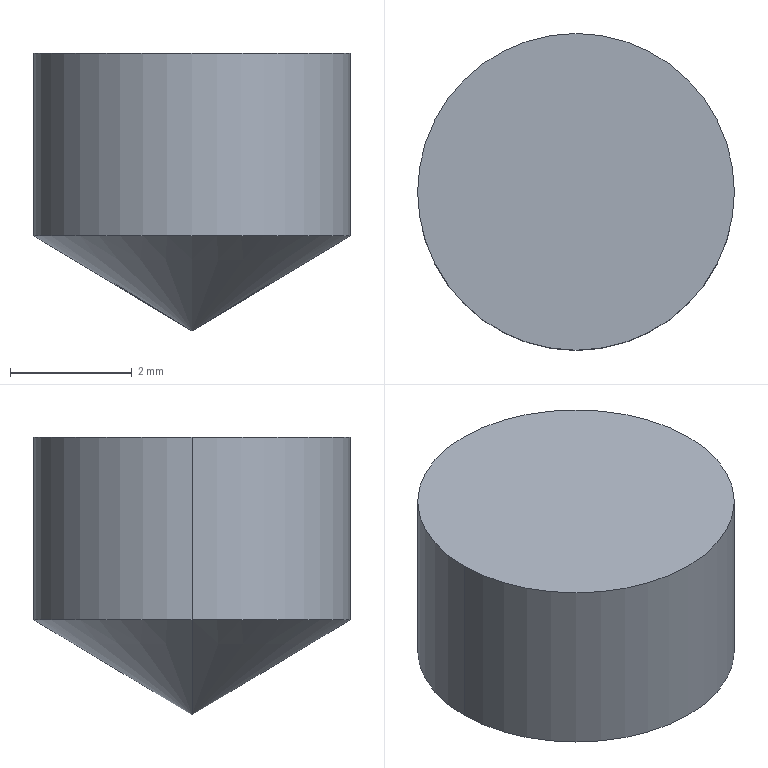Part | SolidWorks | features BaseBody 1 | 1 solid | 5 faces | box 5.2 x 5.2 x 4.562 mm | volume 74.771 mm3 | cylinder 2 | cone 2 | plane 1 | commonest cylinder face diameters 5.2 x2
STEP:
#1=CARTESIAN_POINT('',(-227.35,-157.5,81.));
#2=VERTEX_POINT('',#1);
#3=CARTESIAN_POINT('',(-222.15,-157.5,81.));
#4=VERTEX_POINT('',#3);
#5=CARTESIAN_POINT('',(-224.75,-157.5,81.));
#6=DIRECTION('',(0.,0.,-1.));
#7=DIRECTION('',(-1.,0.,0.));
#8=AXIS2_PLACEMENT_3D('',#5,#6,#7);
#9=CIRCLE('',#8,2.6);
#10=EDGE_CURVE('',#2,#4,#9,.T.);
#11=ORIENTED_EDGE('',*,*,#10,.T.);
#12=CARTESIAN_POINT('',(-222.15,-157.5,78.));
#13=VERTEX_POINT('',#12);
#14=CARTESIAN_POINT('',(-222.15,-157.5,94.));
#15=DIRECTION('',(0.,0.,-1.));
#16=VECTOR('',#15,1000.);
#17=LINE('',#14,#16);
#18=EDGE_CURVE('',#4,#13,#17,.T.);
#19=ORIENTED_EDGE('',*,*,#18,.T.);
#20=CARTESIAN_POINT('',(-227.35,-157.5,78.));
#21=VERTEX_POINT('',#20);
#22=CARTESIAN_POINT('',(-224.75,-157.5,78.));
#23=DIRECTION('',(0.,0.,1.));
#24=DIRECTION('',(-1.,0.,0.));
#25=AXIS2_PLACEMENT_3D('',#22,#23,#24);
#26=CIRCLE('',#25,2.6);
#27=EDGE_CURVE('',#13,#21,#26,.T.);
#28=ORIENTED_EDGE('',*,*,#27,.T.);
#29=CARTESIAN_POINT('',(-227.35,-157.5,94.));
#30=DIRECTION('',(0.,0.,-1.));
#31=VECTOR('',#30,1000.);
#32=LINE('',#29,#31);
#33=EDGE_CURVE('',#2,#21,#32,.T.);
#34=ORIENTED_EDGE('',*,*,#33,.F.);
#35=EDGE_LOOP('',(#11,#19,#28,#34));
#36=FACE_OUTER_BOUND('',#35,.T.);
#37=CARTESIAN_POINT('',(-224.75,-157.5,94.));
#38=DIRECTION('',(0.,0.,-1.));
#39=DIRECTION('',(-1.,0.,0.));
#40=AXIS2_PLACEMENT_3D('',#37,#38,#39);
#41=CYLINDRICAL_SURFACE('',#40,2.6);
#42=ADVANCED_FACE('',(#36),#41,.T.);
#43=CARTESIAN_POINT('',(-224.75,-157.5,76.438));
#44=VERTEX_POINT('',#43);
#45=CARTESIAN_POINT('',(-222.15,-157.5,78.));
#46=DIRECTION('',(0.8572,0.,0.515));
#47=VECTOR('',#46,1000.);
#48=LINE('',#45,#47);
#49=EDGE_CURVE('',#44,#13,#48,.T.);
#50=ORIENTED_EDGE('',*,*,#49,.F.);
#51=CARTESIAN_POINT('',(-227.35,-157.5,78.));
#52=DIRECTION('',(-0.8572,0.,0.515));
#53=VECTOR('',#52,1000.);
#54=LINE('',#51,#53);
#55=EDGE_CURVE('',#44,#21,#54,.T.);
#56=ORIENTED_EDGE('',*,*,#55,.T.);
#57=ORIENTED_EDGE('',*,*,#27,.F.);
#58=EDGE_LOOP('',(#50,#56,#57));
#59=FACE_OUTER_BOUND('',#58,.T.);
#60=CARTESIAN_POINT('',(-224.75,-157.5,78.));
#61=DIRECTION('',(0.,0.,1.));
#62=DIRECTION('',(1.,0.,0.));
#63=AXIS2_PLACEMENT_3D('',#60,#61,#62);
#64=CONICAL_SURFACE('',#63,2.6,1.03);
#65=ADVANCED_FACE('',(#59),#64,.T.);
#66=ORIENTED_EDGE('',*,*,#10,.F.);
#67=CARTESIAN_POINT('',(-224.75,-157.5,81.));
#68=DIRECTION('',(0.,0.,-1.));
#69=DIRECTION('',(-1.,0.,0.));
#70=AXIS2_PLACEMENT_3D('',#67,#68,#69);
#71=CIRCLE('',#70,2.6);
#72=EDGE_CURVE('',#4,#2,#71,.T.);
#73=ORIENTED_EDGE('',*,*,#72,.F.);
#74=EDGE_LOOP('',(#66,#73));
#75=FACE_OUTER_BOUND('',#74,.T.);
#76=CARTESIAN_POINT('',(-221.9,-4.,81.));
#77=DIRECTION('',(0.,0.,1.));
#78=DIRECTION('',(1.,0.,0.));
#79=AXIS2_PLACEMENT_3D('',#76,#77,#78);
#80=PLANE('',#79);
#81=ADVANCED_FACE('',(#75),#80,.T.);
#82=ORIENTED_EDGE('',*,*,#55,.F.);
#83=ORIENTED_EDGE('',*,*,#49,.T.);
#84=CARTESIAN_POINT('',(-224.75,-157.5,78.));
#85=DIRECTION('',(0.,0.,1.));
#86=DIRECTION('',(-1.,0.,0.));
#87=AXIS2_PLACEMENT_3D('',#84,#85,#86);
#88=CIRCLE('',#87,2.6);
#89=EDGE_CURVE('',#21,#13,#88,.T.);
#90=ORIENTED_EDGE('',*,*,#89,.F.);
#91=EDGE_LOOP('',(#82,#83,#90));
#92=FACE_OUTER_BOUND('',#91,.T.);
#93=CARTESIAN_POINT('',(-224.75,-157.5,78.));
#94=DIRECTION('',(0.,0.,1.));
#95=DIRECTION('',(1.,0.,0.));
#96=AXIS2_PLACEMENT_3D('',#93,#94,#95);
#97=CONICAL_SURFACE('',#96,2.6,1.03);
#98=ADVANCED_FACE('',(#92),#97,.T.);
#99=ORIENTED_EDGE('',*,*,#18,.F.);
#100=ORIENTED_EDGE('',*,*,#72,.T.);
#101=ORIENTED_EDGE('',*,*,#33,.T.);
#102=ORIENTED_EDGE('',*,*,#89,.T.);
#103=EDGE_LOOP('',(#99,#100,#101,#102));
#104=FACE_OUTER_BOUND('',#103,.T.);
#105=CARTESIAN_POINT('',(-224.75,-157.5,94.));
#106=DIRECTION('',(0.,0.,-1.));
#107=DIRECTION('',(-1.,0.,0.));
#108=AXIS2_PLACEMENT_3D('',#105,#106,#107);
#109=CYLINDRICAL_SURFACE('',#108,2.6);
#110=ADVANCED_FACE('',(#104),#109,.T.);
#111=CLOSED_SHELL('',(#42,#65,#81,#98,#110));
#112=MANIFOLD_SOLID_BREP('',#111);
#113=CARTESIAN_POINT('',(0.,0.,0.));
#114=DIRECTION('',(0.,0.,1.));
#115=DIRECTION('',(1.,0.,0.));
#116=AXIS2_PLACEMENT_3D('',#113,#114,#115);
#117=(LENGTH_UNIT()NAMED_UNIT(*)SI_UNIT(.MILLI.,.METRE.));
#118=UNCERTAINTY_MEASURE_WITH_UNIT(LENGTH_MEASURE(0.00001),#117,'','');
#119=(NAMED_UNIT(*)PLANE_ANGLE_UNIT()SI_UNIT($,.RADIAN.));
#120=(NAMED_UNIT(*)SI_UNIT($,.STERADIAN.)SOLID_ANGLE_UNIT());
#121=(GEOMETRIC_REPRESENTATION_CONTEXT(3)GLOBAL_UNCERTAINTY_ASSIGNED_CONTEXT((#118))GLOBAL_UNIT_ASSIGNED_CONTEXT((#117,#119,#120))REPRESENTATION_CONTEXT('',''));
#122=ADVANCED_BREP_SHAPE_REPRESENTATION('',(#112,#116),#121);